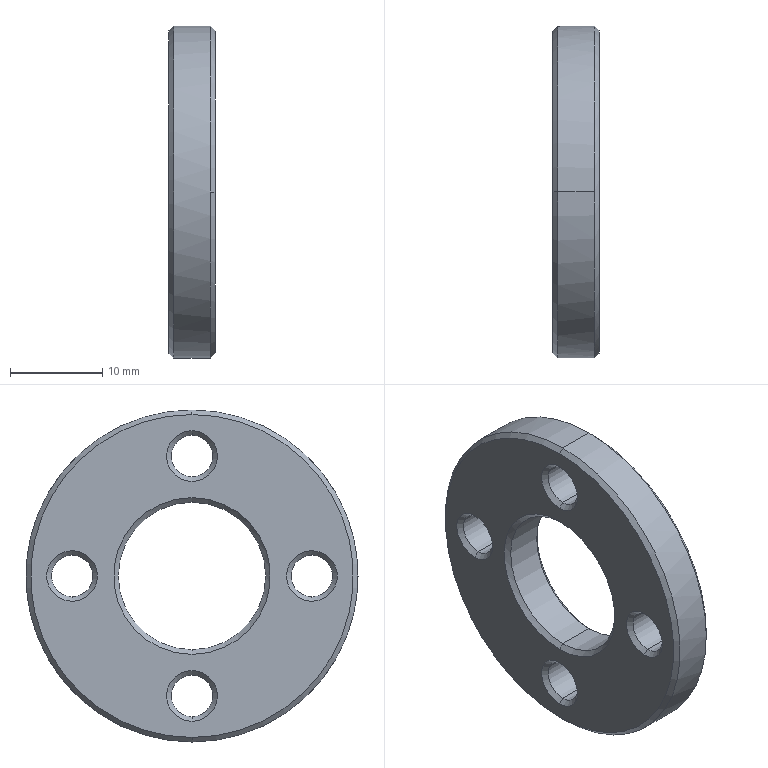Part | STEP file | 03-04 Bearing cover plate | 1 solid | 38 faces | box 5 x 36 x 36 mm | volume 3710 mm3 | cone 24 | cylinder 12 | plane 2 | commonest cylinder face diameters 4.5 x8 16 x2 36 x2